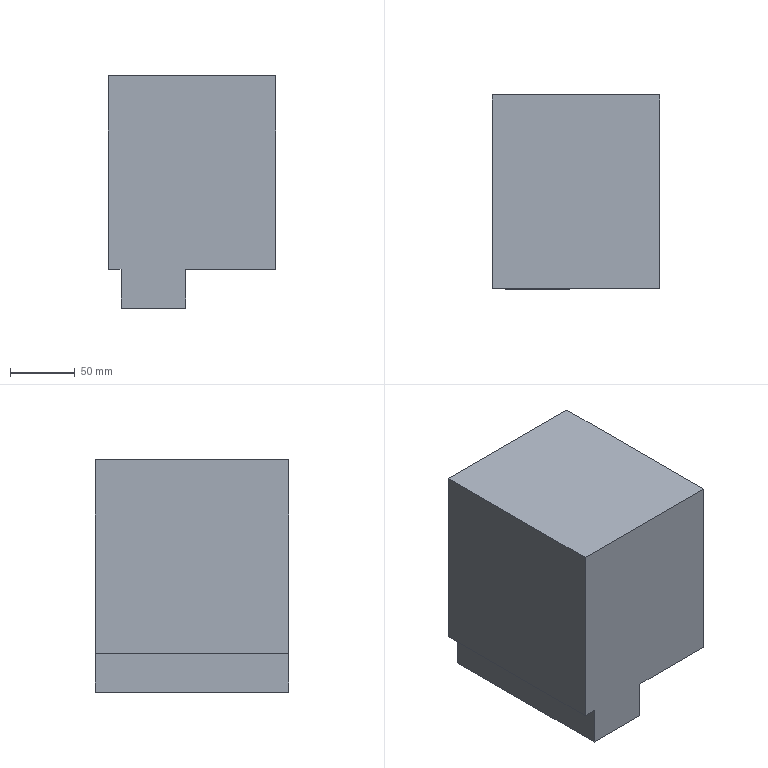Part | SolidWorks | features Extrusion 1 | 1 solid | 10 faces | box 130 x 150 x 180 mm | volume 3150000 mm3 | plane 10
STEP:
#1=CARTESIAN_POINT('',(0.,0.,-150.));
#2=VERTEX_POINT('',#1);
#3=CARTESIAN_POINT('',(0.,0.,0.));
#4=VERTEX_POINT('',#3);
#5=CARTESIAN_POINT('',(0.,0.,-150.));
#6=DIRECTION('',(0.,0.,1.));
#7=VECTOR('',#6,1000.);
#8=LINE('',#5,#7);
#9=EDGE_CURVE('',#2,#4,#8,.T.);
#10=ORIENTED_EDGE('',*,*,#9,.T.);
#11=CARTESIAN_POINT('',(0.,150.,0.));
#12=VERTEX_POINT('',#11);
#13=CARTESIAN_POINT('',(0.,150.,0.));
#14=DIRECTION('',(0.,-1.,0.));
#15=VECTOR('',#14,1000.);
#16=LINE('',#13,#15);
#17=EDGE_CURVE('',#12,#4,#16,.T.);
#18=ORIENTED_EDGE('',*,*,#17,.F.);
#19=CARTESIAN_POINT('',(0.,150.,-150.));
#20=VERTEX_POINT('',#19);
#21=CARTESIAN_POINT('',(0.,150.,-150.));
#22=DIRECTION('',(0.,0.,1.));
#23=VECTOR('',#22,1000.);
#24=LINE('',#21,#23);
#25=EDGE_CURVE('',#20,#12,#24,.T.);
#26=ORIENTED_EDGE('',*,*,#25,.F.);
#27=CARTESIAN_POINT('',(0.,150.,-150.));
#28=DIRECTION('',(0.,-1.,0.));
#29=VECTOR('',#28,1000.);
#30=LINE('',#27,#29);
#31=EDGE_CURVE('',#20,#2,#30,.T.);
#32=ORIENTED_EDGE('',*,*,#31,.T.);
#33=EDGE_LOOP('',(#10,#18,#26,#32));
#34=FACE_OUTER_BOUND('',#33,.T.);
#35=CARTESIAN_POINT('',(0.,150.,-150.));
#36=DIRECTION('',(1.,0.,0.));
#37=DIRECTION('',(0.,0.,-1.));
#38=AXIS2_PLACEMENT_3D('',#35,#36,#37);
#39=PLANE('',#38);
#40=ADVANCED_FACE('',(#34),#39,.F.);
#41=CARTESIAN_POINT('',(130.,0.,0.));
#42=VERTEX_POINT('',#41);
#43=CARTESIAN_POINT('',(0.,0.,0.));
#44=DIRECTION('',(1.,0.,0.));
#45=VECTOR('',#44,1000.);
#46=LINE('',#43,#45);
#47=EDGE_CURVE('',#4,#42,#46,.T.);
#48=ORIENTED_EDGE('',*,*,#47,.T.);
#49=CARTESIAN_POINT('',(130.,150.,0.));
#50=VERTEX_POINT('',#49);
#51=CARTESIAN_POINT('',(130.,150.,0.));
#52=DIRECTION('',(0.,-1.,0.));
#53=VECTOR('',#52,1000.);
#54=LINE('',#51,#53);
#55=EDGE_CURVE('',#50,#42,#54,.T.);
#56=ORIENTED_EDGE('',*,*,#55,.F.);
#57=CARTESIAN_POINT('',(0.,150.,0.));
#58=DIRECTION('',(1.,0.,0.));
#59=VECTOR('',#58,1000.);
#60=LINE('',#57,#59);
#61=EDGE_CURVE('',#12,#50,#60,.T.);
#62=ORIENTED_EDGE('',*,*,#61,.F.);
#63=ORIENTED_EDGE('',*,*,#17,.T.);
#64=EDGE_LOOP('',(#48,#56,#62,#63));
#65=FACE_OUTER_BOUND('',#64,.T.);
#66=CARTESIAN_POINT('',(0.,150.,0.));
#67=DIRECTION('',(0.,0.,-1.));
#68=DIRECTION('',(-1.,0.,0.));
#69=AXIS2_PLACEMENT_3D('',#66,#67,#68);
#70=PLANE('',#69);
#71=ADVANCED_FACE('',(#65),#70,.F.);
#72=CARTESIAN_POINT('',(130.,0.,-150.));
#73=VERTEX_POINT('',#72);
#74=CARTESIAN_POINT('',(130.,0.,0.));
#75=DIRECTION('',(0.,0.,-1.));
#76=VECTOR('',#75,1000.);
#77=LINE('',#74,#76);
#78=EDGE_CURVE('',#42,#73,#77,.T.);
#79=ORIENTED_EDGE('',*,*,#78,.T.);
#80=CARTESIAN_POINT('',(130.,150.,-150.));
#81=VERTEX_POINT('',#80);
#82=CARTESIAN_POINT('',(130.,150.,-150.));
#83=DIRECTION('',(0.,-1.,0.));
#84=VECTOR('',#83,1000.);
#85=LINE('',#82,#84);
#86=EDGE_CURVE('',#81,#73,#85,.T.);
#87=ORIENTED_EDGE('',*,*,#86,.F.);
#88=CARTESIAN_POINT('',(130.,150.,0.));
#89=DIRECTION('',(0.,0.,-1.));
#90=VECTOR('',#89,1000.);
#91=LINE('',#88,#90);
#92=EDGE_CURVE('',#50,#81,#91,.T.);
#93=ORIENTED_EDGE('',*,*,#92,.F.);
#94=ORIENTED_EDGE('',*,*,#55,.T.);
#95=EDGE_LOOP('',(#79,#87,#93,#94));
#96=FACE_OUTER_BOUND('',#95,.T.);
#97=CARTESIAN_POINT('',(130.,150.,0.));
#98=DIRECTION('',(-1.,0.,0.));
#99=DIRECTION('',(0.,0.,1.));
#100=AXIS2_PLACEMENT_3D('',#97,#98,#99);
#101=PLANE('',#100);
#102=ADVANCED_FACE('',(#96),#101,.F.);
#103=CARTESIAN_POINT('',(60.,0.,-150.));
#104=VERTEX_POINT('',#103);
#105=CARTESIAN_POINT('',(130.,0.,-150.));
#106=DIRECTION('',(-1.,0.,0.));
#107=VECTOR('',#106,1000.);
#108=LINE('',#105,#107);
#109=EDGE_CURVE('',#73,#104,#108,.T.);
#110=ORIENTED_EDGE('',*,*,#109,.T.);
#111=CARTESIAN_POINT('',(60.,150.,-150.));
#112=VERTEX_POINT('',#111);
#113=CARTESIAN_POINT('',(60.,150.,-150.));
#114=DIRECTION('',(0.,-1.,0.));
#115=VECTOR('',#114,1000.);
#116=LINE('',#113,#115);
#117=EDGE_CURVE('',#112,#104,#116,.T.);
#118=ORIENTED_EDGE('',*,*,#117,.F.);
#119=CARTESIAN_POINT('',(130.,150.,-150.));
#120=DIRECTION('',(-1.,0.,0.));
#121=VECTOR('',#120,1000.);
#122=LINE('',#119,#121);
#123=EDGE_CURVE('',#81,#112,#122,.T.);
#124=ORIENTED_EDGE('',*,*,#123,.F.);
#125=ORIENTED_EDGE('',*,*,#86,.T.);
#126=EDGE_LOOP('',(#110,#118,#124,#125));
#127=FACE_OUTER_BOUND('',#126,.T.);
#128=CARTESIAN_POINT('',(130.,150.,-150.));
#129=DIRECTION('',(0.,0.,1.));
#130=DIRECTION('',(1.,0.,0.));
#131=AXIS2_PLACEMENT_3D('',#128,#129,#130);
#132=PLANE('',#131);
#133=ADVANCED_FACE('',(#127),#132,.F.);
#134=CARTESIAN_POINT('',(60.,0.,-180.));
#135=VERTEX_POINT('',#134);
#136=CARTESIAN_POINT('',(60.,0.,-150.));
#137=DIRECTION('',(0.,0.,-1.));
#138=VECTOR('',#137,1000.);
#139=LINE('',#136,#138);
#140=EDGE_CURVE('',#104,#135,#139,.T.);
#141=ORIENTED_EDGE('',*,*,#140,.T.);
#142=CARTESIAN_POINT('',(60.,150.,-180.));
#143=VERTEX_POINT('',#142);
#144=CARTESIAN_POINT('',(60.,150.,-180.));
#145=DIRECTION('',(0.,-1.,0.));
#146=VECTOR('',#145,1000.);
#147=LINE('',#144,#146);
#148=EDGE_CURVE('',#143,#135,#147,.T.);
#149=ORIENTED_EDGE('',*,*,#148,.F.);
#150=CARTESIAN_POINT('',(60.,150.,-150.));
#151=DIRECTION('',(0.,0.,-1.));
#152=VECTOR('',#151,1000.);
#153=LINE('',#150,#152);
#154=EDGE_CURVE('',#112,#143,#153,.T.);
#155=ORIENTED_EDGE('',*,*,#154,.F.);
#156=ORIENTED_EDGE('',*,*,#117,.T.);
#157=EDGE_LOOP('',(#141,#149,#155,#156));
#158=FACE_OUTER_BOUND('',#157,.T.);
#159=CARTESIAN_POINT('',(60.,150.,-150.));
#160=DIRECTION('',(-1.,0.,0.));
#161=DIRECTION('',(0.,0.,1.));
#162=AXIS2_PLACEMENT_3D('',#159,#160,#161);
#163=PLANE('',#162);
#164=ADVANCED_FACE('',(#158),#163,.F.);
#165=CARTESIAN_POINT('',(10.,0.,-180.));
#166=VERTEX_POINT('',#165);
#167=CARTESIAN_POINT('',(60.,0.,-180.));
#168=DIRECTION('',(-1.,0.,0.));
#169=VECTOR('',#168,1000.);
#170=LINE('',#167,#169);
#171=EDGE_CURVE('',#135,#166,#170,.T.);
#172=ORIENTED_EDGE('',*,*,#171,.T.);
#173=CARTESIAN_POINT('',(10.,150.,-180.));
#174=VERTEX_POINT('',#173);
#175=CARTESIAN_POINT('',(10.,150.,-180.));
#176=DIRECTION('',(0.,-1.,0.));
#177=VECTOR('',#176,1000.);
#178=LINE('',#175,#177);
#179=EDGE_CURVE('',#174,#166,#178,.T.);
#180=ORIENTED_EDGE('',*,*,#179,.F.);
#181=CARTESIAN_POINT('',(60.,150.,-180.));
#182=DIRECTION('',(-1.,0.,0.));
#183=VECTOR('',#182,1000.);
#184=LINE('',#181,#183);
#185=EDGE_CURVE('',#143,#174,#184,.T.);
#186=ORIENTED_EDGE('',*,*,#185,.F.);
#187=ORIENTED_EDGE('',*,*,#148,.T.);
#188=EDGE_LOOP('',(#172,#180,#186,#187));
#189=FACE_OUTER_BOUND('',#188,.T.);
#190=CARTESIAN_POINT('',(60.,150.,-180.));
#191=DIRECTION('',(0.,0.,1.));
#192=DIRECTION('',(1.,0.,0.));
#193=AXIS2_PLACEMENT_3D('',#190,#191,#192);
#194=PLANE('',#193);
#195=ADVANCED_FACE('',(#189),#194,.F.);
#196=CARTESIAN_POINT('',(10.,0.,-150.));
#197=VERTEX_POINT('',#196);
#198=CARTESIAN_POINT('',(10.,0.,-180.));
#199=DIRECTION('',(0.,0.,1.));
#200=VECTOR('',#199,1000.);
#201=LINE('',#198,#200);
#202=EDGE_CURVE('',#166,#197,#201,.T.);
#203=ORIENTED_EDGE('',*,*,#202,.T.);
#204=CARTESIAN_POINT('',(10.,150.,-150.));
#205=VERTEX_POINT('',#204);
#206=CARTESIAN_POINT('',(10.,150.,-150.));
#207=DIRECTION('',(0.,-1.,0.));
#208=VECTOR('',#207,1000.);
#209=LINE('',#206,#208);
#210=EDGE_CURVE('',#205,#197,#209,.T.);
#211=ORIENTED_EDGE('',*,*,#210,.F.);
#212=CARTESIAN_POINT('',(10.,150.,-180.));
#213=DIRECTION('',(0.,0.,1.));
#214=VECTOR('',#213,1000.);
#215=LINE('',#212,#214);
#216=EDGE_CURVE('',#174,#205,#215,.T.);
#217=ORIENTED_EDGE('',*,*,#216,.F.);
#218=ORIENTED_EDGE('',*,*,#179,.T.);
#219=EDGE_LOOP('',(#203,#211,#217,#218));
#220=FACE_OUTER_BOUND('',#219,.T.);
#221=CARTESIAN_POINT('',(10.,150.,-180.));
#222=DIRECTION('',(1.,0.,0.));
#223=DIRECTION('',(0.,0.,-1.));
#224=AXIS2_PLACEMENT_3D('',#221,#222,#223);
#225=PLANE('',#224);
#226=ADVANCED_FACE('',(#220),#225,.F.);
#227=CARTESIAN_POINT('',(10.,0.,-150.));
#228=DIRECTION('',(-1.,0.,0.));
#229=VECTOR('',#228,1000.);
#230=LINE('',#227,#229);
#231=EDGE_CURVE('',#197,#2,#230,.T.);
#232=ORIENTED_EDGE('',*,*,#231,.T.);
#233=ORIENTED_EDGE('',*,*,#31,.F.);
#234=CARTESIAN_POINT('',(10.,150.,-150.));
#235=DIRECTION('',(-1.,0.,0.));
#236=VECTOR('',#235,1000.);
#237=LINE('',#234,#236);
#238=EDGE_CURVE('',#205,#20,#237,.T.);
#239=ORIENTED_EDGE('',*,*,#238,.F.);
#240=ORIENTED_EDGE('',*,*,#210,.T.);
#241=EDGE_LOOP('',(#232,#233,#239,#240));
#242=FACE_OUTER_BOUND('',#241,.T.);
#243=CARTESIAN_POINT('',(10.,150.,-150.));
#244=DIRECTION('',(0.,0.,1.));
#245=DIRECTION('',(1.,0.,0.));
#246=AXIS2_PLACEMENT_3D('',#243,#244,#245);
#247=PLANE('',#246);
#248=ADVANCED_FACE('',(#242),#247,.F.);
#249=ORIENTED_EDGE('',*,*,#25,.T.);
#250=ORIENTED_EDGE('',*,*,#61,.T.);
#251=ORIENTED_EDGE('',*,*,#92,.T.);
#252=ORIENTED_EDGE('',*,*,#123,.T.);
#253=ORIENTED_EDGE('',*,*,#154,.T.);
#254=ORIENTED_EDGE('',*,*,#185,.T.);
#255=ORIENTED_EDGE('',*,*,#216,.T.);
#256=ORIENTED_EDGE('',*,*,#238,.T.);
#257=EDGE_LOOP('',(#249,#250,#251,#252,#253,#254,#255,#256));
#258=FACE_OUTER_BOUND('',#257,.T.);
#259=CARTESIAN_POINT('',(0.,150.,0.));
#260=DIRECTION('',(0.,1.,0.));
#261=DIRECTION('',(0.,0.,1.));
#262=AXIS2_PLACEMENT_3D('',#259,#260,#261);
#263=PLANE('',#262);
#264=ADVANCED_FACE('',(#258),#263,.T.);
#265=ORIENTED_EDGE('',*,*,#9,.F.);
#266=ORIENTED_EDGE('',*,*,#231,.F.);
#267=ORIENTED_EDGE('',*,*,#202,.F.);
#268=ORIENTED_EDGE('',*,*,#171,.F.);
#269=ORIENTED_EDGE('',*,*,#140,.F.);
#270=ORIENTED_EDGE('',*,*,#109,.F.);
#271=ORIENTED_EDGE('',*,*,#78,.F.);
#272=ORIENTED_EDGE('',*,*,#47,.F.);
#273=EDGE_LOOP('',(#265,#266,#267,#268,#269,#270,#271,#272));
#274=FACE_OUTER_BOUND('',#273,.T.);
#275=CARTESIAN_POINT('',(0.,0.,0.));
#276=DIRECTION('',(0.,1.,0.));
#277=DIRECTION('',(0.,0.,1.));
#278=AXIS2_PLACEMENT_3D('',#275,#276,#277);
#279=PLANE('',#278);
#280=ADVANCED_FACE('',(#274),#279,.F.);
#281=CLOSED_SHELL('',(#40,#71,#102,#133,#164,#195,#226,#248,#264,#280));
#282=MANIFOLD_SOLID_BREP('',#281);
#283=CARTESIAN_POINT('',(0.,0.,0.));
#284=DIRECTION('',(0.,0.,1.));
#285=DIRECTION('',(1.,0.,0.));
#286=AXIS2_PLACEMENT_3D('',#283,#284,#285);
#287=(LENGTH_UNIT()NAMED_UNIT(*)SI_UNIT(.MILLI.,.METRE.));
#288=UNCERTAINTY_MEASURE_WITH_UNIT(LENGTH_MEASURE(0.00001),#287,'','');
#289=(NAMED_UNIT(*)PLANE_ANGLE_UNIT()SI_UNIT($,.RADIAN.));
#290=(NAMED_UNIT(*)SI_UNIT($,.STERADIAN.)SOLID_ANGLE_UNIT());
#291=(GEOMETRIC_REPRESENTATION_CONTEXT(3)GLOBAL_UNCERTAINTY_ASSIGNED_CONTEXT((#288))GLOBAL_UNIT_ASSIGNED_CONTEXT((#287,#289,#290))REPRESENTATION_CONTEXT('',''));
#292=ADVANCED_BREP_SHAPE_REPRESENTATION('',(#282,#286),#291);